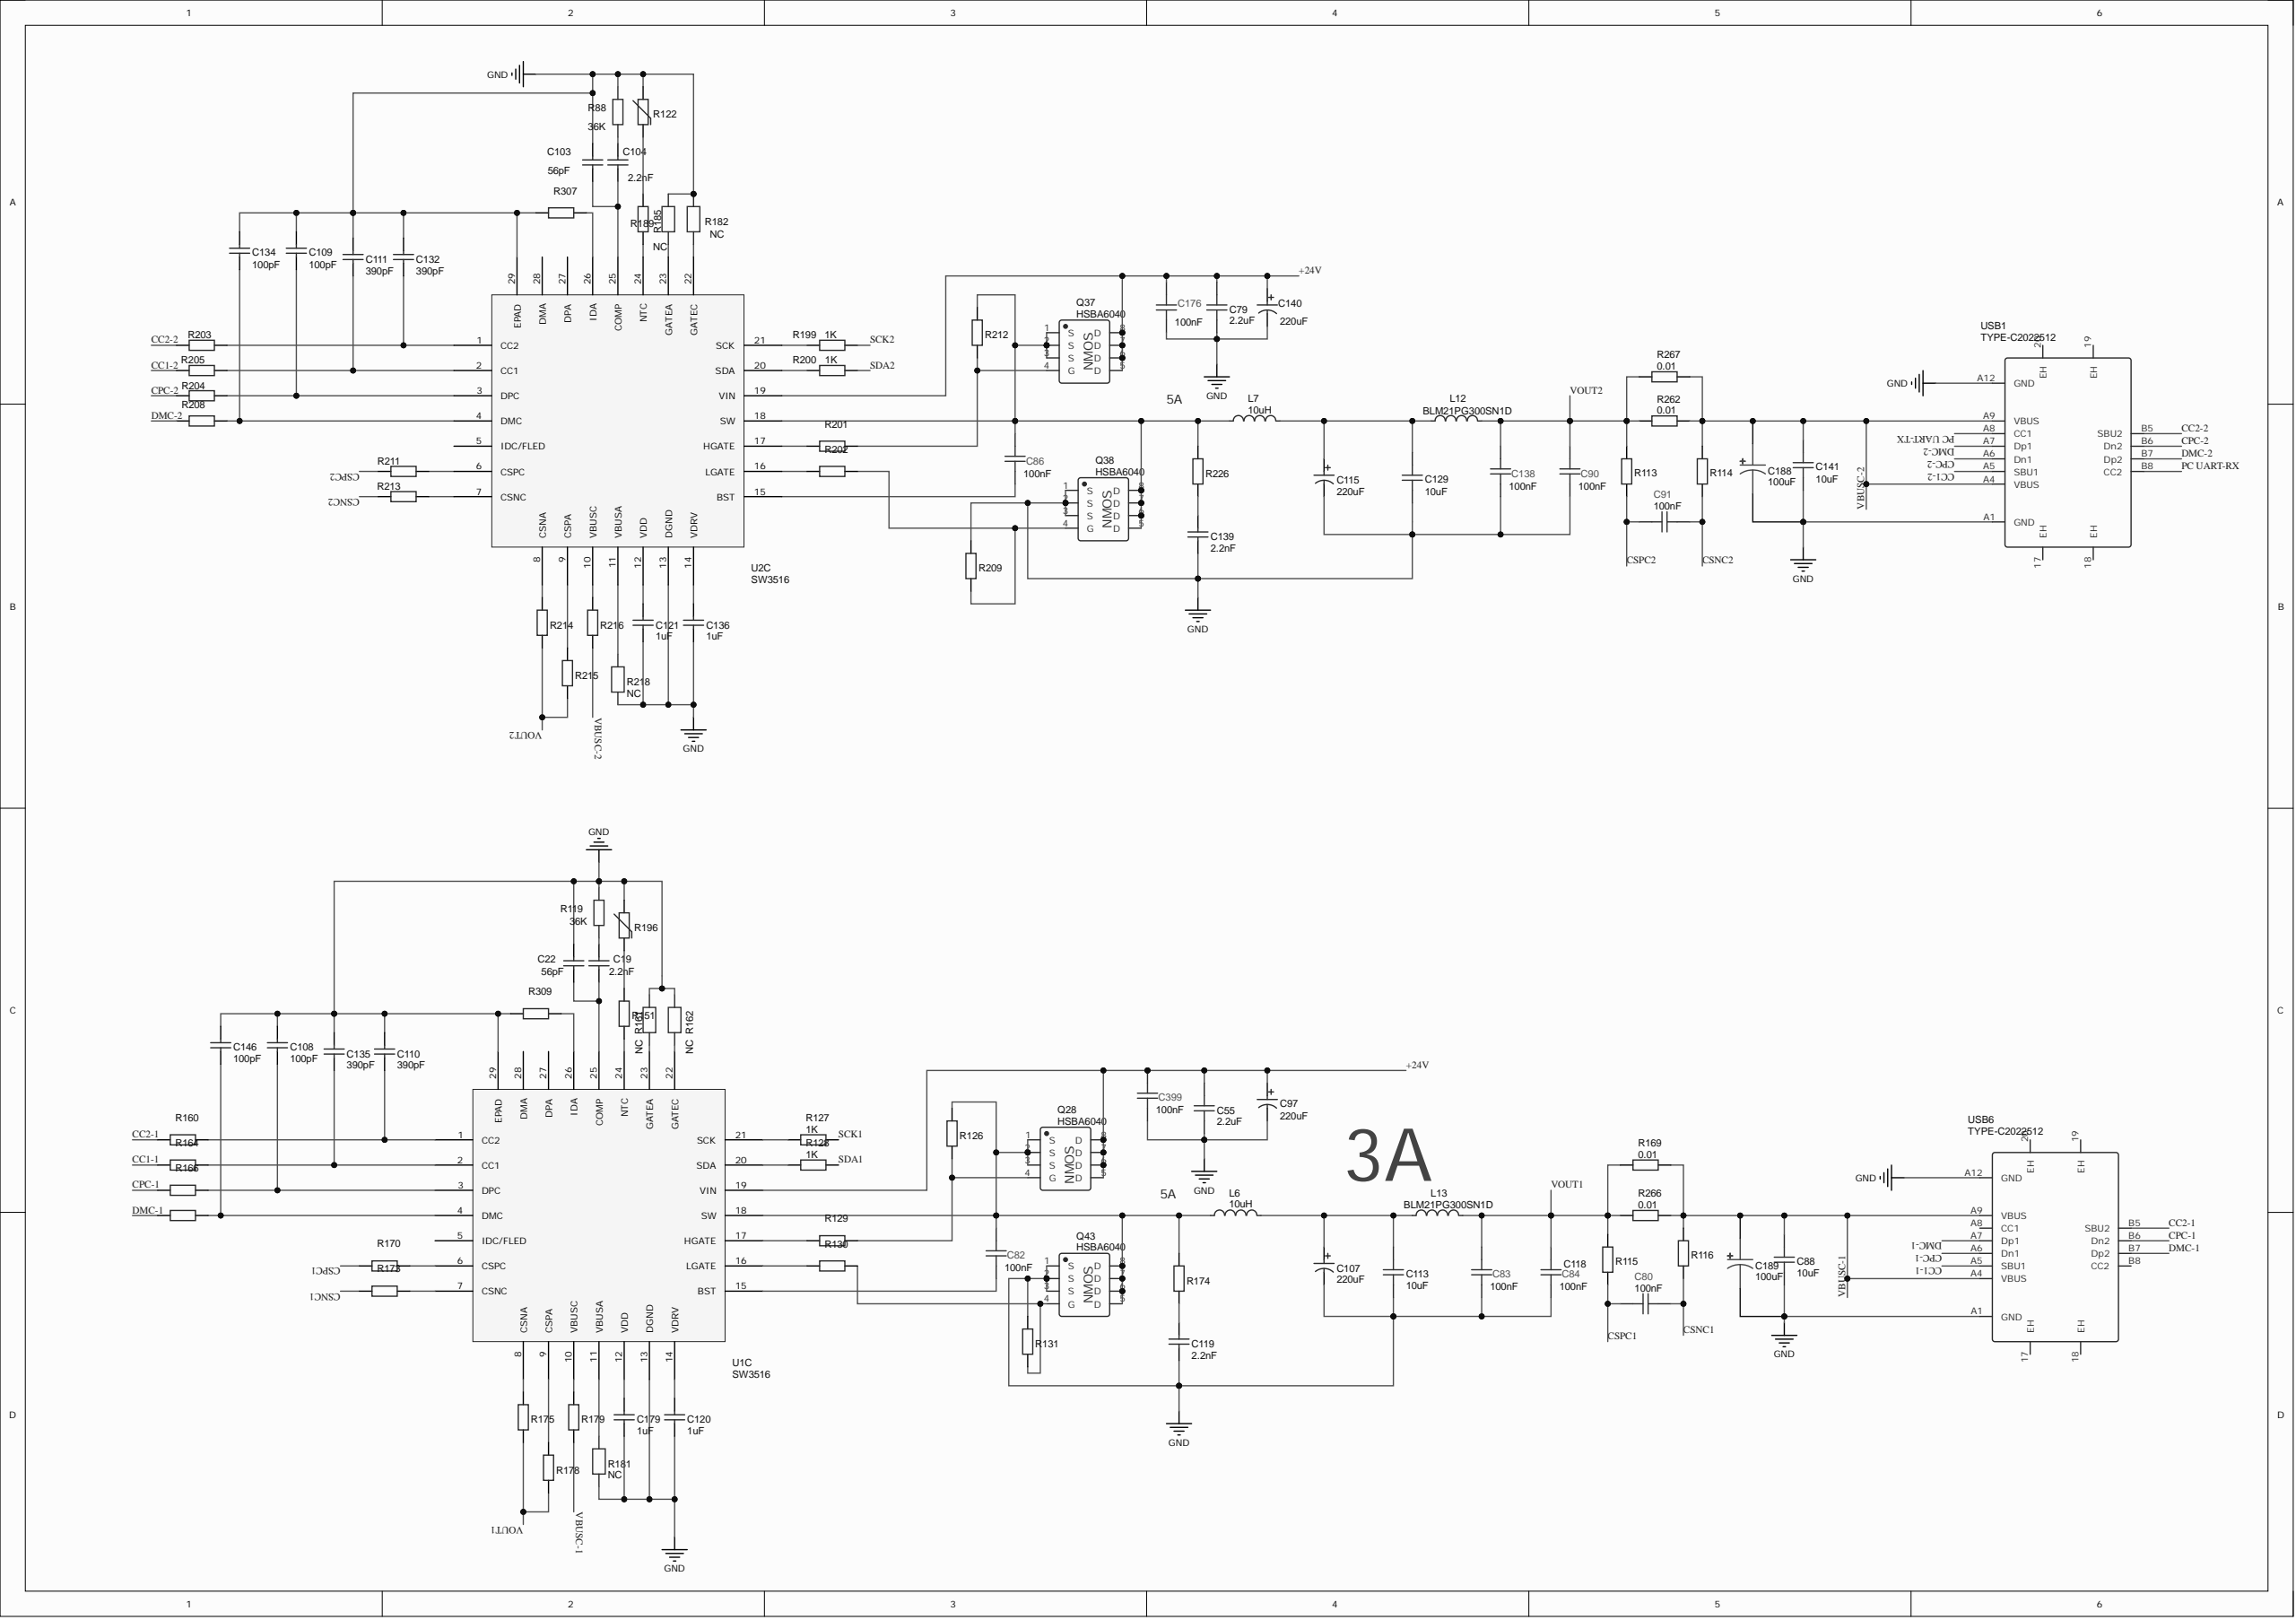Circuit board | Altium Designer | 694 parts | 423 nets | one sheet of the schematic
Parts on this sheet (reference | value | footprint):
C19 | 2.2nF | C0603
C22 | 56pF | C0603
C55 | 2.2uF | C0603
C79 | 2.2uF | C0603
C80 | 100nF | C0603
C82 | 100nF | C0603
C83 | 100nF | C0603
C84 | 100nF | C0603
C86 | 100nF | C0603
C88 | 10uF | C0603
C90 | 100nF | C0603
C91 | 100nF | C0603
C97 | 220uF | CAP-TH_BD8.0-P3.50-D0.6-FD
C103 | 56pF | C0603
C104 | 2.2nF | C0603
C107 | 220uF | CAP-TH_BD8.0-P3.50-D0.6-FD
C108 | 100pF | C0603
C109 | 100pF | C0603
C110 | 390pF | C0603
C111 | 390pF | C0603
C113 | 10uF | C0603
C115 | 220uF | CAP-TH_BD8.0-P3.50-D0.6-FD
C119 | 2.2nF | C0603
C120 | 1uF | C0603
C121 | 1uF | C0603
C129 | 10uF | C0603
C132 | 390pF | C0603
C134 | 100pF | C0603
C135 | 390pF | C0603
C136 | 1uF | C0603
C138 | 100nF | C0603
C139 | 2.2nF | C0603
C140 | 220uF | CAP-TH_BD8.0-P3.50-D0.6-FD
C141 | 10uF | C0603
C146 | 100pF | C0603
C176 | 100nF | C0603
C179 | 1uF | C0603
C188 | 100uF | CAP-TH_BD6.3-P2.50-D1.0-FD
C189 | 100uF | CAP-TH_BD6.3-P2.50-D1.0-FD
C399 | 100nF | C0603
L6 | 10uH | IND-SMD_L13.8-W12.6_YSPI13XX
L7 | 10uH | IND-SMD_L13.8-W12.6_YSPI13XX
L12 | BLM21PG300SN1D | L0805
L13 | BLM21PG300SN1D | L0805
Q28 | HSBA6040 | POWERPAK-SO-8_L6.2-W5.2-P1.27-BR-EP
Q37 | HSBA6040 | POWERPAK-SO-8_L6.2-W5.2-P1.27-BR-EP
Q38 | HSBA6040 | POWERPAK-SO-8_L6.2-W5.2-P1.27-BR-EP
Q43 | HSBA6040 | POWERPAK-SO-8_L6.2-W5.2-P1.27-BR-EP
R88 | 36K | R0603
R113 | R0603
R114 | R0603
R115 | R0603
R116 | R0603
R119 | 36K | R0603
R122 | R0603
R126 | R0603
R127 | 1K | R0603
R128 | 1K | R0603
R129 | R0603
R130 | R0603
R131 | R0603
R151 | R0603
R160 | R0603
R161 | NC | R0603
R162 | NC | R0603
R164 | R0603
R166 | R0603
R169 | 0.01 | R2512
R170 | R0603
R173 | R0603
R174 | R0603
R175 | R0603
R178 | R0603
R179 | R0603
R181 | NC | R0603
R182 | NC | R0603
R185 | NC | R0603
R189 | R0603
R196 | R0603
R199 | 1K | R0603
R200 | 1K | R0603
R201 | R0603
R202 | R0603
R203 | R0603
R204 | R0603
R205 | R0603
R208 | R0603
R209 | R0603
R211 | R0603
R212 | R0603
R213 | R0603
R214 | R0603
R215 | R0603
R216 | R0603
R218 | NC | R0603
R226 | R0603
R262 | 0.01 | R2512
R266 | 0.01 | R2512
R267 | 0.01 | R2512
R307 | R0603
R309 | R0603
U1 | LM5116MHX | HTSSOP-20_L6.5-W4.4-P0.65-LS6.4-BL-EP
U1C | =value | QFN-28_L4.0-W4.0-P0.40-BL-EP
U2C | =value | QFN-28_L4.0-W4.0-P0.40-BL-EP
USB1 | TYPE-C2022512 | NEW_TYPEC
USB6 | TYPE-C2022512 | NEW_TYPEC
Nets of these parts (net: part-pin ...):
VOUT2: C90-2 C138-2 L12-2 R113-2 R214-1 R215-1 R262-1 R267-1
VOUT1: C83-2 C84-2 L13-2 R115-2 R169-1 R175-1 R178-1 R266-1
VBUSC-2: C141-2 C188-1 R114-2 R216-1 R262-2 R267-2 USB1-A4 USB1-A9
VBUSC-1: C88-2 C189-1 R116-2 R169-2 R179-1 R266-2 USB6-A4 USB6-A9
SDA2: R200-2
SDA1: R128-2
SCK2: R199-2
SCK1: R127-2
PC UART-TX: USB1-A8
PC UART-RX: USB1-B8
NetR309_2: R309-2 U1C-26
NetR307_2: R307-2 U2C-26
NetR218_1: R218-1 U2C-11
NetR216_2: R216-2 U2C-10
NetR215_2: R215-2 U2C-9
NetR214_2: R214-2 U2C-8
NetR213_2: R213-2 U2C-7
NetR211_2: R211-2 U2C-6
NetR202_1: R202-1 U2C-16
NetR201_1: R201-1 U2C-17
NetR200_1: R200-1 U2C-20
NetR199_1: R199-1 U2C-21
NetR189_1: R189-1 U2C-24
NetR185_1: R185-1 U2C-23
NetR182_1: R182-1 U2C-22
NetR181_1: R181-1 U1C-11
NetR179_2: R179-2 U1C-10
NetR178_2: R178-2 U1C-9
NetR175_2: R175-2 U1C-8
NetR173_2: R173-2 U1C-7
NetR170_2: R170-2 U1C-6
NetR162_1: R162-1 U1C-22
NetR161_1: R161-1 U1C-23
NetR151_2: R151-2 R196-1
NetR151_1: R151-1 U1C-24
NetR130_1: R130-1 U1C-16
NetR129_1: R129-1 U1C-17
NetR128_1: R128-1 U1C-20
NetR127_1: R127-1 U1C-21
NetR122_1: R122-1 R189-2
NetQ43_4: Q43-4 R130-2 R131-1
NetQ38_4: Q38-4 R202-2 R209-1
NetQ37_4: Q37-4 R201-2 R212-1
NetQ28_4: Q28-4 R126-1 R129-2
NetC179_2: C179-2 U1C-12
NetC146_1: C146-1 U1C-4
NetC139_2: C139-2 R226-1
NetC136_2: C136-2 U2C-14
NetC135_1: C135-1 R164-2 U1C-2
NetC134_1: C134-1 R208-2 U2C-4
NetC132_1: C132-1 R203-2 U2C-1
NetC121_2: C121-2 U2C-12
NetC120_2: C120-2 U1C-14
NetC119_2: C119-2 R174-1
NetC115_1: C115-1 C129-2 L7-2 L12-1
NetC111_1: C111-1 R205-2 U2C-2
NetC110_1: C110-1 R160-2 U1C-1
NetC109_1: C109-1 R204-2 U2C-3
NetC108_1: C108-1 R166-2 U1C-3
NetC107_1: C107-1 C113-2 L6-2 L13-1
NetC104_2: C104-2 R88-1
NetC103_2: C103-2 C104-1 U2C-25
NetC86_2: C86-2 L7-1 Q37-1 Q37-2 Q37-3 Q38-5 Q38-6 Q38-7 Q38-8 R212-2 R226-2 U2C-18
NetC86_1: C86-1 U2C-15
NetC82_2: C82-2 L6-1 Q28-1 Q28-2 Q28-3 Q43-5 Q43-6 Q43-7 Q43-8 R126-2 R174-2 U1C-18
NetC82_1: C82-1 U1C-15
NetC19_2: C19-2 R119-1
NetC19_1: C19-1 C22-1 U1C-25
GND: C22-2 C55-1 C79-1 C83-1 C84-1 C88-1 C90-1 C97-2 C103-1 C107-2 C108-2 C109-2 C110-2 C111-2 C113-1 C115-2 C119-1 C120-1 C121-1 C129-1 C132-2 C134-2 C135-2 C136-1 C138-1 C139-1 C140-2 C141-1 C146-2 C176-1 C179-1 C188-2 C189-2 C399-1 Q38-1 Q38-2 Q38-3 Q43-1 Q43-2 Q43-3 R88-2 R119-2 R122-2 R131-2 R161-2 R162-2 R181-2 R182-2 R185-2 R196-2 R209-2 R218-2 R307-1 R309-1 USB1-A1 USB1-A12 USB6-A1 USB6-A12 U1-6 U1-14 U1-21 U1C-13 U1C-29 U2C-13 U2C-29
DMC-2: R208-1 USB1-A7 USB1-B7
DMC-1: USB6-A7 USB6-B7
CSPC2: C91-2 R113-1 R211-1
CSPC1: C80-2 R115-1 R170-1
CSNC2: C91-1 R114-1 R213-1
CSNC1: C80-1 R116-1 R173-1
CPC-2: R204-1 USB1-A6 USB1-B6
CPC-1: R166-1 USB6-A6 USB6-B6
CC2-2: R203-1 USB1-B5
CC2-1: R160-1 USB6-B5
CC1-2: R205-1 USB1-A5
CC1-1: R164-1 USB6-A5
+24V: C55-2 C79-2 C97-1 C140-1 C176-2 C399-2 Q28-5 Q28-6 Q28-7 Q28-8 Q37-5 Q37-6 Q37-7 Q37-8 U1-10 U1C-19 U2C-19